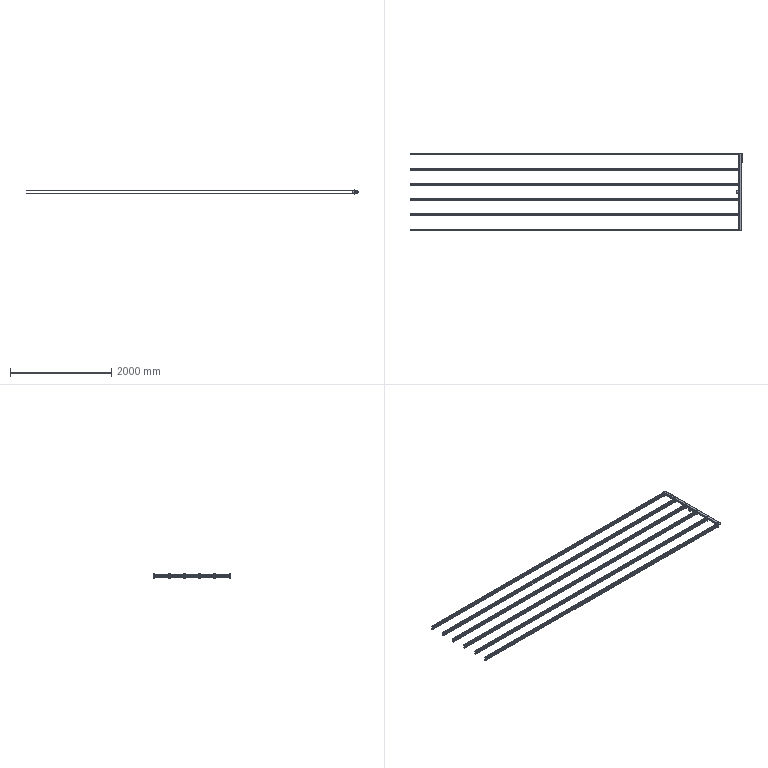Part | SolidWorks | features ReferencePattern 111, LocalLPattern 3 | 27 solids | 1620 faces | box 6573 x 1530 x 100 mm | volume 13010460 mm3 | cylinder 1380 | plane 214 | cone 26 | commonest cylinder face diameters 13 x1152 4 x48 8 x48 10 x36 6 x28 6.8 x24